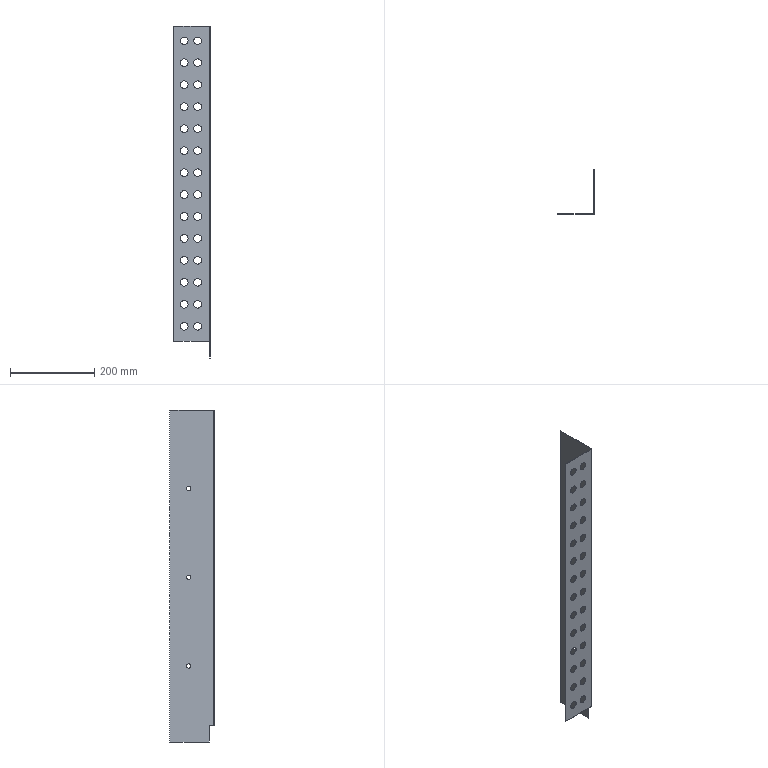Part | STEP file | 68379539 | 1 solid | 82 faces | box 86.7 x 104.75 x 786 mm | volume 103690 mm3 | cylinder 64 | plane 18 | commonest cylinder face diameters 18 x56 10 x6 1.6 x1 3.1 x1